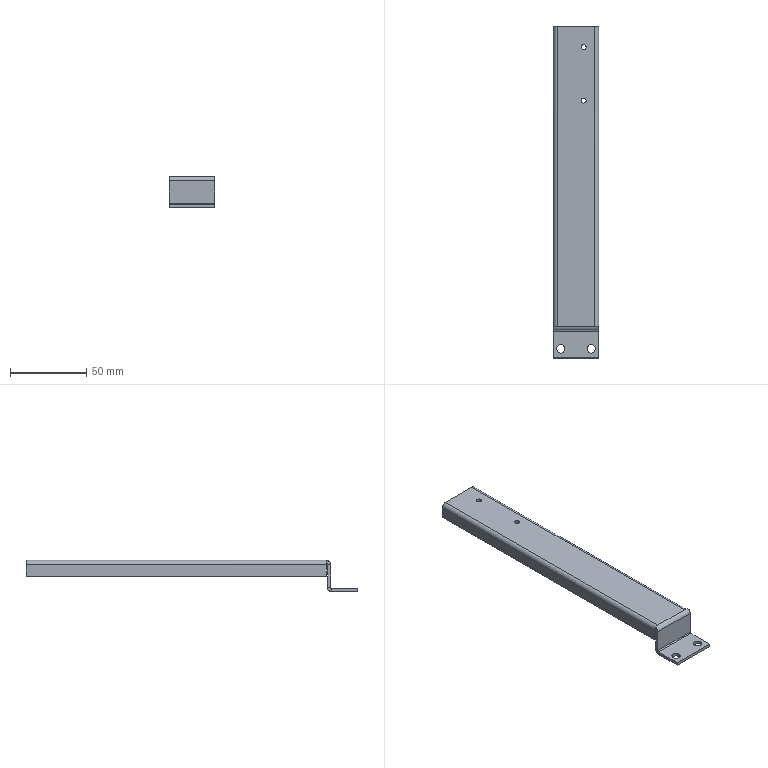Part | SolidWorks | features EdgeFlange 3, FlatPattern 1, HoleWzd 1, ICE 1, SMBaseFlange 1, SheetMetal 1 | 1 solid | 48 faces | box 30 x 218 x 20.5 mm | volume 20090 mm3 | plane 32 | cylinder 16 | commonest cylinder face diameters 1.473 x4 3.3 x4 5.473 x4 5.5 x4
STEP:
#1=CARTESIAN_POINT('',(3.35,194.,16.5));
#2=VERTEX_POINT('',#1);
#3=CARTESIAN_POINT('',(6.65,194.,16.5));
#4=VERTEX_POINT('',#3);
#5=CARTESIAN_POINT('',(5.,194.,16.5));
#6=DIRECTION('',(0.,0.,1.));
#7=DIRECTION('',(0.,-1.,0.));
#8=AXIS2_PLACEMENT_3D('',#5,#6,#7);
#9=CIRCLE('',#8,1.65);
#10=EDGE_CURVE('',#2,#4,#9,.T.);
#11=ORIENTED_EDGE('',*,*,#10,.F.);
#12=CARTESIAN_POINT('',(3.35,194.,18.5));
#13=VERTEX_POINT('',#12);
#14=CARTESIAN_POINT('',(3.35,194.,18.5));
#15=DIRECTION('',(0.,0.,1.));
#16=VECTOR('',#15,1000.);
#17=LINE('',#14,#16);
#18=EDGE_CURVE('',#2,#13,#17,.T.);
#19=ORIENTED_EDGE('',*,*,#18,.T.);
#20=CARTESIAN_POINT('',(6.65,194.,18.5));
#21=VERTEX_POINT('',#20);
#22=CARTESIAN_POINT('',(5.,194.,18.5));
#23=DIRECTION('',(0.,0.,1.));
#24=DIRECTION('',(1.,0.,0.));
#25=AXIS2_PLACEMENT_3D('',#22,#23,#24);
#26=CIRCLE('',#25,1.65);
#27=EDGE_CURVE('',#13,#21,#26,.T.);
#28=ORIENTED_EDGE('',*,*,#27,.T.);
#29=CARTESIAN_POINT('',(6.65,194.,18.5));
#30=DIRECTION('',(0.,0.,1.));
#31=VECTOR('',#30,1000.);
#32=LINE('',#29,#31);
#33=EDGE_CURVE('',#4,#21,#32,.T.);
#34=ORIENTED_EDGE('',*,*,#33,.F.);
#35=EDGE_LOOP('',(#11,#19,#28,#34));
#36=FACE_OUTER_BOUND('',#35,.T.);
#37=CARTESIAN_POINT('',(5.,194.,18.5));
#38=DIRECTION('',(0.,0.,1.));
#39=DIRECTION('',(1.,0.,0.));
#40=AXIS2_PLACEMENT_3D('',#37,#38,#39);
#41=CYLINDRICAL_SURFACE('',#40,1.65);
#42=ADVANCED_FACE('',(#36),#41,.F.);
#43=CARTESIAN_POINT('',(3.35,159.,16.5));
#44=VERTEX_POINT('',#43);
#45=CARTESIAN_POINT('',(6.65,159.,16.5));
#46=VERTEX_POINT('',#45);
#47=CARTESIAN_POINT('',(5.,159.,16.5));
#48=DIRECTION('',(0.,0.,1.));
#49=DIRECTION('',(0.,-1.,0.));
#50=AXIS2_PLACEMENT_3D('',#47,#48,#49);
#51=CIRCLE('',#50,1.65);
#52=EDGE_CURVE('',#44,#46,#51,.T.);
#53=ORIENTED_EDGE('',*,*,#52,.F.);
#54=CARTESIAN_POINT('',(3.35,159.,18.5));
#55=VERTEX_POINT('',#54);
#56=CARTESIAN_POINT('',(3.35,159.,18.5));
#57=DIRECTION('',(0.,0.,1.));
#58=VECTOR('',#57,1000.);
#59=LINE('',#56,#58);
#60=EDGE_CURVE('',#44,#55,#59,.T.);
#61=ORIENTED_EDGE('',*,*,#60,.T.);
#62=CARTESIAN_POINT('',(6.65,159.,18.5));
#63=VERTEX_POINT('',#62);
#64=CARTESIAN_POINT('',(5.,159.,18.5));
#65=DIRECTION('',(0.,0.,1.));
#66=DIRECTION('',(1.,0.,0.));
#67=AXIS2_PLACEMENT_3D('',#64,#65,#66);
#68=CIRCLE('',#67,1.65);
#69=EDGE_CURVE('',#55,#63,#68,.T.);
#70=ORIENTED_EDGE('',*,*,#69,.T.);
#71=CARTESIAN_POINT('',(6.65,159.,18.5));
#72=DIRECTION('',(0.,0.,1.));
#73=VECTOR('',#72,1000.);
#74=LINE('',#71,#73);
#75=EDGE_CURVE('',#46,#63,#74,.T.);
#76=ORIENTED_EDGE('',*,*,#75,.F.);
#77=EDGE_LOOP('',(#53,#61,#70,#76));
#78=FACE_OUTER_BOUND('',#77,.T.);
#79=CARTESIAN_POINT('',(5.,159.,18.5));
#80=DIRECTION('',(0.,0.,1.));
#81=DIRECTION('',(1.,0.,0.));
#82=AXIS2_PLACEMENT_3D('',#79,#80,#81);
#83=CYLINDRICAL_SURFACE('',#82,1.65);
#84=ADVANCED_FACE('',(#78),#83,.F.);
#85=CARTESIAN_POINT('',(7.25,-4.,-2.));
#86=VERTEX_POINT('',#85);
#87=CARTESIAN_POINT('',(12.75,-4.,-2.));
#88=VERTEX_POINT('',#87);
#89=CARTESIAN_POINT('',(10.,-4.,-2.));
#90=DIRECTION('',(0.,0.,1.));
#91=DIRECTION('',(1.,0.,0.));
#92=AXIS2_PLACEMENT_3D('',#89,#90,#91);
#93=CIRCLE('',#92,2.75);
#94=EDGE_CURVE('',#86,#88,#93,.T.);
#95=ORIENTED_EDGE('',*,*,#94,.F.);
#96=CARTESIAN_POINT('',(7.25,-4.,0.));
#97=VERTEX_POINT('',#96);
#98=CARTESIAN_POINT('',(7.25,-4.,-2.));
#99=DIRECTION('',(0.,0.,1.));
#100=VECTOR('',#99,1000.);
#101=LINE('',#98,#100);
#102=EDGE_CURVE('',#86,#97,#101,.T.);
#103=ORIENTED_EDGE('',*,*,#102,.T.);
#104=CARTESIAN_POINT('',(12.75,-4.,0.));
#105=VERTEX_POINT('',#104);
#106=CARTESIAN_POINT('',(10.,-4.,0.));
#107=DIRECTION('',(0.,0.,1.));
#108=DIRECTION('',(1.,0.,0.));
#109=AXIS2_PLACEMENT_3D('',#106,#107,#108);
#110=CIRCLE('',#109,2.75);
#111=EDGE_CURVE('',#97,#105,#110,.T.);
#112=ORIENTED_EDGE('',*,*,#111,.T.);
#113=CARTESIAN_POINT('',(12.75,-4.,-2.));
#114=DIRECTION('',(0.,0.,1.));
#115=VECTOR('',#114,1000.);
#116=LINE('',#113,#115);
#117=EDGE_CURVE('',#88,#105,#116,.T.);
#118=ORIENTED_EDGE('',*,*,#117,.F.);
#119=EDGE_LOOP('',(#95,#103,#112,#118));
#120=FACE_OUTER_BOUND('',#119,.T.);
#121=CARTESIAN_POINT('',(10.,-4.,-2.));
#122=DIRECTION('',(0.,0.,1.));
#123=DIRECTION('',(1.,0.,0.));
#124=AXIS2_PLACEMENT_3D('',#121,#122,#123);
#125=CYLINDRICAL_SURFACE('',#124,2.75);
#126=ADVANCED_FACE('',(#120),#125,.F.);
#127=CARTESIAN_POINT('',(-12.75,-4.,-2.));
#128=VERTEX_POINT('',#127);
#129=CARTESIAN_POINT('',(-7.25,-4.,-2.));
#130=VERTEX_POINT('',#129);
#131=CARTESIAN_POINT('',(-10.,-4.,-2.));
#132=DIRECTION('',(0.,0.,1.));
#133=DIRECTION('',(1.,0.,0.));
#134=AXIS2_PLACEMENT_3D('',#131,#132,#133);
#135=CIRCLE('',#134,2.75);
#136=EDGE_CURVE('',#128,#130,#135,.T.);
#137=ORIENTED_EDGE('',*,*,#136,.F.);
#138=CARTESIAN_POINT('',(-12.75,-4.,0.));
#139=VERTEX_POINT('',#138);
#140=CARTESIAN_POINT('',(-12.75,-4.,-2.));
#141=DIRECTION('',(0.,0.,1.));
#142=VECTOR('',#141,1000.);
#143=LINE('',#140,#142);
#144=EDGE_CURVE('',#128,#139,#143,.T.);
#145=ORIENTED_EDGE('',*,*,#144,.T.);
#146=CARTESIAN_POINT('',(-7.25,-4.,0.));
#147=VERTEX_POINT('',#146);
#148=CARTESIAN_POINT('',(-10.,-4.,0.));
#149=DIRECTION('',(0.,0.,1.));
#150=DIRECTION('',(1.,0.,0.));
#151=AXIS2_PLACEMENT_3D('',#148,#149,#150);
#152=CIRCLE('',#151,2.75);
#153=EDGE_CURVE('',#139,#147,#152,.T.);
#154=ORIENTED_EDGE('',*,*,#153,.T.);
#155=CARTESIAN_POINT('',(-7.25,-4.,-2.));
#156=DIRECTION('',(0.,0.,1.));
#157=VECTOR('',#156,1000.);
#158=LINE('',#155,#157);
#159=EDGE_CURVE('',#130,#147,#158,.T.);
#160=ORIENTED_EDGE('',*,*,#159,.F.);
#161=EDGE_LOOP('',(#137,#145,#154,#160));
#162=FACE_OUTER_BOUND('',#161,.T.);
#163=CARTESIAN_POINT('',(-10.,-4.,-2.));
#164=DIRECTION('',(0.,0.,1.));
#165=DIRECTION('',(1.,0.,0.));
#166=AXIS2_PLACEMENT_3D('',#163,#164,#165);
#167=CYLINDRICAL_SURFACE('',#166,2.75);
#168=ADVANCED_FACE('',(#162),#167,.F.);
#169=CARTESIAN_POINT('',(-15.,10.737,18.5));
#170=VERTEX_POINT('',#169);
#171=CARTESIAN_POINT('',(-12.263,10.737,18.5));
#172=VERTEX_POINT('',#171);
#173=CARTESIAN_POINT('',(0.,10.737,18.5));
#174=DIRECTION('',(1.,0.,0.));
#175=VECTOR('',#174,1000.);
#176=LINE('',#173,#175);
#177=EDGE_CURVE('',#170,#172,#176,.T.);
#178=ORIENTED_EDGE('',*,*,#177,.T.);
#179=CARTESIAN_POINT('',(-14.899,10.737,16.5));
#180=VERTEX_POINT('',#179);
#181=CARTESIAN_POINT('',(-12.263,10.737,15.763));
#182=DIRECTION('',(0.,-1.,0.));
#183=DIRECTION('',(0.,0.,1.));
#184=AXIS2_PLACEMENT_3D('',#181,#182,#183);
#185=CIRCLE('',#184,2.737);
#186=EDGE_CURVE('',#172,#180,#185,.T.);
#187=ORIENTED_EDGE('',*,*,#186,.T.);
#188=CARTESIAN_POINT('',(-15.,10.737,16.5));
#189=VERTEX_POINT('',#188);
#190=CARTESIAN_POINT('',(-15.,10.737,16.5));
#191=DIRECTION('',(1.,0.,0.));
#192=VECTOR('',#191,1000.);
#193=LINE('',#190,#192);
#194=EDGE_CURVE('',#189,#180,#193,.T.);
#195=ORIENTED_EDGE('',*,*,#194,.F.);
#196=CARTESIAN_POINT('',(-15.,10.737,18.5));
#197=DIRECTION('',(0.,0.,1.));
#198=VECTOR('',#197,1000.);
#199=LINE('',#196,#198);
#200=EDGE_CURVE('',#189,#170,#199,.T.);
#201=ORIENTED_EDGE('',*,*,#200,.T.);
#202=EDGE_LOOP('',(#178,#187,#195,#201));
#203=FACE_OUTER_BOUND('',#202,.T.);
#204=CARTESIAN_POINT('',(-12.263,10.737,16.5));
#205=DIRECTION('',(0.,1.,0.));
#206=DIRECTION('',(-1.,0.,0.));
#207=AXIS2_PLACEMENT_3D('',#204,#205,#206);
#208=PLANE('',#207);
#209=ADVANCED_FACE('',(#203),#208,.T.);
#210=CARTESIAN_POINT('',(15.,10.737,16.5));
#211=VERTEX_POINT('',#210);
#212=CARTESIAN_POINT('',(14.899,10.737,16.5));
#213=VERTEX_POINT('',#212);
#214=CARTESIAN_POINT('',(15.,10.737,16.5));
#215=DIRECTION('',(-1.,0.,0.));
#216=VECTOR('',#215,1000.);
#217=LINE('',#214,#216);
#218=EDGE_CURVE('',#211,#213,#217,.T.);
#219=ORIENTED_EDGE('',*,*,#218,.T.);
#220=CARTESIAN_POINT('',(12.263,10.737,18.5));
#221=VERTEX_POINT('',#220);
#222=CARTESIAN_POINT('',(12.263,10.737,15.763));
#223=DIRECTION('',(0.,-1.,0.));
#224=DIRECTION('',(0.,0.,-1.));
#225=AXIS2_PLACEMENT_3D('',#222,#223,#224);
#226=CIRCLE('',#225,2.737);
#227=EDGE_CURVE('',#213,#221,#226,.T.);
#228=ORIENTED_EDGE('',*,*,#227,.T.);
#229=CARTESIAN_POINT('',(15.,10.737,18.5));
#230=VERTEX_POINT('',#229);
#231=CARTESIAN_POINT('',(0.,10.737,18.5));
#232=DIRECTION('',(-1.,0.,0.));
#233=VECTOR('',#232,1000.);
#234=LINE('',#231,#233);
#235=EDGE_CURVE('',#230,#221,#234,.T.);
#236=ORIENTED_EDGE('',*,*,#235,.F.);
#237=CARTESIAN_POINT('',(15.,10.737,16.5));
#238=DIRECTION('',(0.,0.,1.));
#239=VECTOR('',#238,1000.);
#240=LINE('',#237,#239);
#241=EDGE_CURVE('',#211,#230,#240,.T.);
#242=ORIENTED_EDGE('',*,*,#241,.F.);
#243=EDGE_LOOP('',(#219,#228,#236,#242));
#244=FACE_OUTER_BOUND('',#243,.T.);
#245=CARTESIAN_POINT('',(15.,10.737,16.5));
#246=DIRECTION('',(0.,1.,0.));
#247=DIRECTION('',(-1.,0.,0.));
#248=AXIS2_PLACEMENT_3D('',#245,#246,#247);
#249=PLANE('',#248);
#250=ADVANCED_FACE('',(#244),#249,.T.);
#251=CARTESIAN_POINT('',(5.,194.,18.5));
#252=DIRECTION('',(0.,0.,1.));
#253=DIRECTION('',(1.,0.,0.));
#254=AXIS2_PLACEMENT_3D('',#251,#252,#253);
#255=CIRCLE('',#254,1.65);
#256=EDGE_CURVE('',#21,#13,#255,.T.);
#257=ORIENTED_EDGE('',*,*,#256,.F.);
#258=ORIENTED_EDGE('',*,*,#27,.F.);
#259=EDGE_LOOP('',(#257,#258));
#260=FACE_BOUND('',#259,.T.);
#261=CARTESIAN_POINT('',(5.,159.,18.5));
#262=DIRECTION('',(0.,0.,1.));
#263=DIRECTION('',(1.,0.,0.));
#264=AXIS2_PLACEMENT_3D('',#261,#262,#263);
#265=CIRCLE('',#264,1.65);
#266=EDGE_CURVE('',#63,#55,#265,.T.);
#267=ORIENTED_EDGE('',*,*,#266,.F.);
#268=ORIENTED_EDGE('',*,*,#69,.F.);
#269=EDGE_LOOP('',(#267,#268));
#270=FACE_BOUND('',#269,.T.);
#271=CARTESIAN_POINT('',(-12.263,208.,18.5));
#272=VERTEX_POINT('',#271);
#273=CARTESIAN_POINT('',(12.263,208.,18.5));
#274=VERTEX_POINT('',#273);
#275=CARTESIAN_POINT('',(15.,208.,18.5));
#276=DIRECTION('',(1.,0.,0.));
#277=VECTOR('',#276,1000.);
#278=LINE('',#275,#277);
#279=EDGE_CURVE('',#272,#274,#278,.T.);
#280=ORIENTED_EDGE('',*,*,#279,.F.);
#281=CARTESIAN_POINT('',(-12.263,208.,18.5));
#282=DIRECTION('',(0.,-1.,0.));
#283=VECTOR('',#282,1000.);
#284=LINE('',#281,#283);
#285=EDGE_CURVE('',#272,#172,#284,.T.);
#286=ORIENTED_EDGE('',*,*,#285,.T.);
#287=CARTESIAN_POINT('',(0.,10.737,18.5));
#288=DIRECTION('',(1.,0.,0.));
#289=VECTOR('',#288,1000.);
#290=LINE('',#287,#289);
#291=EDGE_CURVE('',#172,#221,#290,.T.);
#292=ORIENTED_EDGE('',*,*,#291,.T.);
#293=CARTESIAN_POINT('',(12.263,10.737,18.5));
#294=DIRECTION('',(0.,1.,0.));
#295=VECTOR('',#294,1000.);
#296=LINE('',#293,#295);
#297=EDGE_CURVE('',#221,#274,#296,.T.);
#298=ORIENTED_EDGE('',*,*,#297,.T.);
#299=EDGE_LOOP('',(#280,#286,#292,#298));
#300=FACE_OUTER_BOUND('',#299,.T.);
#301=CARTESIAN_POINT('',(0.,0.,18.5));
#302=DIRECTION('',(0.,0.,1.));
#303=DIRECTION('',(0.,-1.,0.));
#304=AXIS2_PLACEMENT_3D('',#301,#302,#303);
#305=PLANE('',#304);
#306=ADVANCED_FACE('',(#260,#270,#300),#305,.T.);
#307=CARTESIAN_POINT('',(5.,194.,16.5));
#308=DIRECTION('',(0.,0.,1.));
#309=DIRECTION('',(0.,-1.,0.));
#310=AXIS2_PLACEMENT_3D('',#307,#308,#309);
#311=CIRCLE('',#310,1.65);
#312=EDGE_CURVE('',#4,#2,#311,.T.);
#313=ORIENTED_EDGE('',*,*,#312,.T.);
#314=ORIENTED_EDGE('',*,*,#10,.T.);
#315=EDGE_LOOP('',(#313,#314));
#316=FACE_BOUND('',#315,.T.);
#317=CARTESIAN_POINT('',(5.,159.,16.5));
#318=DIRECTION('',(0.,0.,1.));
#319=DIRECTION('',(0.,-1.,0.));
#320=AXIS2_PLACEMENT_3D('',#317,#318,#319);
#321=CIRCLE('',#320,1.65);
#322=EDGE_CURVE('',#46,#44,#321,.T.);
#323=ORIENTED_EDGE('',*,*,#322,.T.);
#324=ORIENTED_EDGE('',*,*,#52,.T.);
#325=EDGE_LOOP('',(#323,#324));
#326=FACE_BOUND('',#325,.T.);
#327=CARTESIAN_POINT('',(-12.263,208.,16.5));
#328=VERTEX_POINT('',#327);
#329=CARTESIAN_POINT('',(-12.263,10.737,16.5));
#330=VERTEX_POINT('',#329);
#331=CARTESIAN_POINT('',(-12.263,208.,16.5));
#332=DIRECTION('',(0.,-1.,0.));
#333=VECTOR('',#332,1000.);
#334=LINE('',#331,#333);
#335=EDGE_CURVE('',#328,#330,#334,.T.);
#336=ORIENTED_EDGE('',*,*,#335,.F.);
#337=CARTESIAN_POINT('',(12.263,208.,16.5));
#338=VERTEX_POINT('',#337);
#339=CARTESIAN_POINT('',(0.,208.,16.5));
#340=DIRECTION('',(1.,0.,0.));
#341=VECTOR('',#340,1000.);
#342=LINE('',#339,#341);
#343=EDGE_CURVE('',#328,#338,#342,.T.);
#344=ORIENTED_EDGE('',*,*,#343,.T.);
#345=CARTESIAN_POINT('',(12.263,10.737,16.5));
#346=VERTEX_POINT('',#345);
#347=CARTESIAN_POINT('',(12.263,10.737,16.5));
#348=DIRECTION('',(0.,1.,0.));
#349=VECTOR('',#348,1000.);
#350=LINE('',#347,#349);
#351=EDGE_CURVE('',#346,#338,#350,.T.);
#352=ORIENTED_EDGE('',*,*,#351,.F.);
#353=CARTESIAN_POINT('',(-15.,10.737,16.5));
#354=DIRECTION('',(1.,0.,0.));
#355=VECTOR('',#354,1000.);
#356=LINE('',#353,#355);
#357=EDGE_CURVE('',#330,#346,#356,.T.);
#358=ORIENTED_EDGE('',*,*,#357,.F.);
#359=EDGE_LOOP('',(#336,#344,#352,#358));
#360=FACE_OUTER_BOUND('',#359,.T.);
#361=CARTESIAN_POINT('',(0.,0.,16.5));
#362=DIRECTION('',(0.,0.,1.));
#363=DIRECTION('',(0.,-1.,0.));
#364=AXIS2_PLACEMENT_3D('',#361,#362,#363);
#365=PLANE('',#364);
#366=ADVANCED_FACE('',(#316,#326,#360),#365,.F.);
#367=ORIENTED_EDGE('',*,*,#343,.F.);
#368=CARTESIAN_POINT('',(-12.263,208.,16.5));
#369=DIRECTION('',(0.,0.,1.));
#370=VECTOR('',#369,1000.);
#371=LINE('',#368,#370);
#372=EDGE_CURVE('',#328,#272,#371,.T.);
#373=ORIENTED_EDGE('',*,*,#372,.T.);
#374=ORIENTED_EDGE('',*,*,#279,.T.);
#375=CARTESIAN_POINT('',(12.263,208.,16.5));
#376=DIRECTION('',(0.,0.,1.));
#377=VECTOR('',#376,1000.);
#378=LINE('',#375,#377);
#379=EDGE_CURVE('',#338,#274,#378,.T.);
#380=ORIENTED_EDGE('',*,*,#379,.F.);
#381=EDGE_LOOP('',(#367,#373,#374,#380));
#382=FACE_OUTER_BOUND('',#381,.T.);
#383=CARTESIAN_POINT('',(15.,208.,18.5));
#384=DIRECTION('',(0.,1.,0.));
#385=DIRECTION('',(0.,0.,1.));
#386=AXIS2_PLACEMENT_3D('',#383,#384,#385);
#387=PLANE('',#386);
#388=ADVANCED_FACE('',(#382),#387,.T.);
#389=CARTESIAN_POINT('',(15.,10.,0.7366));
#390=VERTEX_POINT('',#389);
#391=CARTESIAN_POINT('',(15.,10.,15.763));
#392=VERTEX_POINT('',#391);
#393=CARTESIAN_POINT('',(15.,10.,18.5));
#394=DIRECTION('',(0.,0.,1.));
#395=VECTOR('',#394,1000.);
#396=LINE('',#393,#395);
#397=EDGE_CURVE('',#390,#392,#396,.T.);
#398=ORIENTED_EDGE('',*,*,#397,.T.);
#399=CARTESIAN_POINT('',(15.,8.,15.763));
#400=VERTEX_POINT('',#399);
#401=CARTESIAN_POINT('',(15.,10.,15.763));
#402=DIRECTION('',(0.,-1.,0.));
#403=VECTOR('',#402,1000.);
#404=LINE('',#401,#403);
#405=EDGE_CURVE('',#392,#400,#404,.T.);
#406=ORIENTED_EDGE('',*,*,#405,.T.);
#407=CARTESIAN_POINT('',(15.,8.,0.7366));
#408=VERTEX_POINT('',#407);
#409=CARTESIAN_POINT('',(15.,8.,0.));
#410=DIRECTION('',(0.,0.,1.));
#411=VECTOR('',#410,1000.);
#412=LINE('',#409,#411);
#413=EDGE_CURVE('',#408,#400,#412,.T.);
#414=ORIENTED_EDGE('',*,*,#413,.F.);
#415=CARTESIAN_POINT('',(15.,10.,0.7366));
#416=DIRECTION('',(0.,1.,0.));
#417=VECTOR('',#416,1000.);
#418=LINE('',#415,#417);
#419=EDGE_CURVE('',#408,#390,#418,.T.);
#420=ORIENTED_EDGE('',*,*,#419,.T.);
#421=EDGE_LOOP('',(#398,#406,#414,#420));
#422=FACE_OUTER_BOUND('',#421,.T.);
#423=CARTESIAN_POINT('',(15.,10.,18.5));
#424=DIRECTION('',(1.,0.,0.));
#425=DIRECTION('',(0.,1.,0.));
#426=AXIS2_PLACEMENT_3D('',#423,#424,#425);
#427=PLANE('',#426);
#428=ADVANCED_FACE('',(#422),#427,.T.);
#429=CARTESIAN_POINT('',(-15.,10.,15.763));
#430=VERTEX_POINT('',#429);
#431=CARTESIAN_POINT('',(-15.,10.,0.7366));
#432=VERTEX_POINT('',#431);
#433=CARTESIAN_POINT('',(-15.,10.,0.));
#434=DIRECTION('',(0.,0.,-1.));
#435=VECTOR('',#434,1000.);
#436=LINE('',#433,#435);
#437=EDGE_CURVE('',#430,#432,#436,.T.);
#438=ORIENTED_EDGE('',*,*,#437,.F.);
#439=CARTESIAN_POINT('',(15.,10.,15.763));
#440=DIRECTION('',(-1.,0.,0.));
#441=VECTOR('',#440,1000.);
#442=LINE('',#439,#441);
#443=EDGE_CURVE('',#392,#430,#442,.T.);
#444=ORIENTED_EDGE('',*,*,#443,.F.);
#445=ORIENTED_EDGE('',*,*,#397,.F.);
#446=CARTESIAN_POINT('',(0.,10.,0.7366));
#447=DIRECTION('',(-1.,0.,0.));
#448=VECTOR('',#447,1000.);
#449=LINE('',#446,#448);
#450=EDGE_CURVE('',#390,#432,#449,.T.);
#451=ORIENTED_EDGE('',*,*,#450,.T.);
#452=EDGE_LOOP('',(#438,#444,#445,#451));
#453=FACE_OUTER_BOUND('',#452,.T.);
#454=CARTESIAN_POINT('',(0.,10.,0.));
#455=DIRECTION('',(0.,1.,0.));
#456=DIRECTION('',(0.,0.,1.));
#457=AXIS2_PLACEMENT_3D('',#454,#455,#456);
#458=PLANE('',#457);
#459=ADVANCED_FACE('',(#453),#458,.T.);
#460=CARTESIAN_POINT('',(-15.,8.,15.763));
#461=VERTEX_POINT('',#460);
#462=CARTESIAN_POINT('',(15.,8.,15.763));
#463=DIRECTION('',(-1.,0.,0.));
#464=VECTOR('',#463,1000.);
#465=LINE('',#462,#464);
#466=EDGE_CURVE('',#400,#461,#465,.T.);
#467=ORIENTED_EDGE('',*,*,#466,.T.);
#468=CARTESIAN_POINT('',(-15.,8.,0.7366));
#469=VERTEX_POINT('',#468);
#470=CARTESIAN_POINT('',(-15.,8.,0.));
#471=DIRECTION('',(0.,0.,-1.));
#472=VECTOR('',#471,1000.);
#473=LINE('',#470,#472);
#474=EDGE_CURVE('',#461,#469,#473,.T.);
#475=ORIENTED_EDGE('',*,*,#474,.T.);
#476=CARTESIAN_POINT('',(15.,8.,0.7366));
#477=DIRECTION('',(-1.,0.,0.));
#478=VECTOR('',#477,1000.);
#479=LINE('',#476,#478);
#480=EDGE_CURVE('',#408,#469,#479,.T.);
#481=ORIENTED_EDGE('',*,*,#480,.F.);
#482=ORIENTED_EDGE('',*,*,#413,.T.);
#483=EDGE_LOOP('',(#467,#475,#481,#482));
#484=FACE_OUTER_BOUND('',#483,.T.);
#485=CARTESIAN_POINT('',(0.,8.,0.));
#486=DIRECTION('',(0.,1.,0.));
#487=DIRECTION('',(0.,0.,1.));
#488=AXIS2_PLACEMENT_3D('',#485,#486,#487);
#489=PLANE('',#488);
#490=ADVANCED_FACE('',(#484),#489,.F.);
#491=CARTESIAN_POINT('',(-15.,7.263,0.));
#492=VERTEX_POINT('',#491);
#493=CARTESIAN_POINT('',(-15.,-10.,0.));
#494=VERTEX_POINT('',#493);
#495=CARTESIAN_POINT('',(-15.,-10.,0.));
#496=DIRECTION('',(0.,-1.,0.));
#497=VECTOR('',#496,1000.);
#498=LINE('',#495,#497);
#499=EDGE_CURVE('',#492,#494,#498,.T.);
#500=ORIENTED_EDGE('',*,*,#499,.F.);
#501=CARTESIAN_POINT('',(-15.,7.263,-2.));
#502=VERTEX_POINT('',#501);
#503=CARTESIAN_POINT('',(-15.,7.263,0.));
#504=DIRECTION('',(0.,0.,-1.));
#505=VECTOR('',#504,1000.);
#506=LINE('',#503,#505);
#507=EDGE_CURVE('',#492,#502,#506,.T.);
#508=ORIENTED_EDGE('',*,*,#507,.T.);
#509=CARTESIAN_POINT('',(-15.,-10.,-2.));
#510=VERTEX_POINT('',#509);
#511=CARTESIAN_POINT('',(-15.,-10.,-2.));
#512=DIRECTION('',(0.,-1.,0.));
#513=VECTOR('',#512,1000.);
#514=LINE('',#511,#513);
#515=EDGE_CURVE('',#502,#510,#514,.T.);
#516=ORIENTED_EDGE('',*,*,#515,.T.);
#517=CARTESIAN_POINT('',(-15.,-10.,-2.));
#518=DIRECTION('',(0.,0.,1.));
#519=VECTOR('',#518,1000.);
#520=LINE('',#517,#519);
#521=EDGE_CURVE('',#510,#494,#520,.T.);
#522=ORIENTED_EDGE('',*,*,#521,.T.);
#523=EDGE_LOOP('',(#500,#508,#516,#522));
#524=FACE_OUTER_BOUND('',#523,.T.);
#525=CARTESIAN_POINT('',(-15.,-10.,-2.));
#526=DIRECTION('',(-1.,0.,0.));
#527=DIRECTION('',(0.,0.,1.));
#528=AXIS2_PLACEMENT_3D('',#525,#526,#527);
#529=PLANE('',#528);
#530=ADVANCED_FACE('',(#524),#529,.T.);
#531=CARTESIAN_POINT('',(10.,-4.,-2.));
#532=DIRECTION('',(0.,0.,1.));
#533=DIRECTION('',(1.,0.,0.));
#534=AXIS2_PLACEMENT_3D('',#531,#532,#533);
#535=CIRCLE('',#534,2.75);
#536=EDGE_CURVE('',#88,#86,#535,.T.);
#537=ORIENTED_EDGE('',*,*,#536,.T.);
#538=ORIENTED_EDGE('',*,*,#94,.T.);
#539=EDGE_LOOP('',(#537,#538));
#540=FACE_BOUND('',#539,.T.);
#541=CARTESIAN_POINT('',(-10.,-4.,-2.));
#542=DIRECTION('',(0.,0.,1.));
#543=DIRECTION('',(1.,0.,0.));
#544=AXIS2_PLACEMENT_3D('',#541,#542,#543);
#545=CIRCLE('',#544,2.75);
#546=EDGE_CURVE('',#130,#128,#545,.T.);
#547=ORIENTED_EDGE('',*,*,#546,.T.);
#548=ORIENTED_EDGE('',*,*,#136,.T.);
#549=EDGE_LOOP('',(#547,#548));
#550=FACE_BOUND('',#549,.T.);
#551=CARTESIAN_POINT('',(15.,7.263,-2.));
#552=VERTEX_POINT('',#551);
#553=CARTESIAN_POINT('',(-15.,7.263,-2.));
#554=DIRECTION('',(1.,0.,0.));
#555=VECTOR('',#554,1000.);
#556=LINE('',#553,#555);
#557=EDGE_CURVE('',#502,#552,#556,.T.);
#558=ORIENTED_EDGE('',*,*,#557,.T.);
#559=CARTESIAN_POINT('',(15.,-10.,-2.));
#560=VERTEX_POINT('',#559);
#561=CARTESIAN_POINT('',(15.,-10.,-2.));
#562=DIRECTION('',(0.,1.,0.));
#563=VECTOR('',#562,1000.);
#564=LINE('',#561,#563);
#565=EDGE_CURVE('',#560,#552,#564,.T.);
#566=ORIENTED_EDGE('',*,*,#565,.F.);
#567=CARTESIAN_POINT('',(15.,-10.,-2.));
#568=DIRECTION('',(1.,0.,0.));
#569=VECTOR('',#568,1000.);
#570=LINE('',#567,#569);
#571=EDGE_CURVE('',#510,#560,#570,.T.);
#572=ORIENTED_EDGE('',*,*,#571,.F.);
#573=ORIENTED_EDGE('',*,*,#515,.F.);
#574=EDGE_LOOP('',(#558,#566,#572,#573));
#575=FACE_OUTER_BOUND('',#574,.T.);
#576=CARTESIAN_POINT('',(0.,0.,-2.));
#577=DIRECTION('',(0.,0.,1.));
#578=DIRECTION('',(1.,0.,0.));
#579=AXIS2_PLACEMENT_3D('',#576,#577,#578);
#580=PLANE('',#579);
#581=ADVANCED_FACE('',(#540,#550,#575),#580,.F.);
#582=CARTESIAN_POINT('',(10.,-4.,0.));
#583=DIRECTION('',(0.,0.,1.));
#584=DIRECTION('',(1.,0.,0.));
#585=AXIS2_PLACEMENT_3D('',#582,#583,#584);
#586=CIRCLE('',#585,2.75);
#587=EDGE_CURVE('',#105,#97,#586,.T.);
#588=ORIENTED_EDGE('',*,*,#587,.F.);
#589=ORIENTED_EDGE('',*,*,#111,.F.);
#590=EDGE_LOOP('',(#588,#589));
#591=FACE_BOUND('',#590,.T.);
#592=CARTESIAN_POINT('',(-10.,-4.,0.));
#593=DIRECTION('',(0.,0.,1.));
#594=DIRECTION('',(1.,0.,0.));
#595=AXIS2_PLACEMENT_3D('',#592,#593,#594);
#596=CIRCLE('',#595,2.75);
#597=EDGE_CURVE('',#147,#139,#596,.T.);
#598=ORIENTED_EDGE('',*,*,#597,.F.);
#599=ORIENTED_EDGE('',*,*,#153,.F.);
#600=EDGE_LOOP('',(#598,#599));
#601=FACE_BOUND('',#600,.T.);
#602=CARTESIAN_POINT('',(15.,-10.,0.));
#603=VERTEX_POINT('',#602);
#604=CARTESIAN_POINT('',(15.,7.263,0.));
#605=VERTEX_POINT('',#604);
#606=CARTESIAN_POINT('',(15.,-10.,0.));
#607=DIRECTION('',(0.,1.,0.));
#608=VECTOR('',#607,1000.);
#609=LINE('',#606,#608);
#610=EDGE_CURVE('',#603,#605,#609,.T.);
#611=ORIENTED_EDGE('',*,*,#610,.T.);
#612=CARTESIAN_POINT('',(-15.,7.263,0.));
#613=DIRECTION('',(1.,0.,0.));
#614=VECTOR('',#613,1000.);
#615=LINE('',#612,#614);
#616=EDGE_CURVE('',#492,#605,#615,.T.);
#617=ORIENTED_EDGE('',*,*,#616,.F.);
#618=ORIENTED_EDGE('',*,*,#499,.T.);
#619=CARTESIAN_POINT('',(15.,-10.,0.));
#620=DIRECTION('',(1.,0.,0.));
#621=VECTOR('',#620,1000.);
#622=LINE('',#619,#621);
#623=EDGE_CURVE('',#494,#603,#622,.T.);
#624=ORIENTED_EDGE('',*,*,#623,.T.);
#625=EDGE_LOOP('',(#611,#617,#618,#624));
#626=FACE_OUTER_BOUND('',#625,.T.);
#627=CARTESIAN_POINT('',(0.,0.,0.));
#628=DIRECTION('',(0.,0.,1.));
#629=DIRECTION('',(1.,0.,0.));
#630=AXIS2_PLACEMENT_3D('',#627,#628,#629);
#631=PLANE('',#630);
#632=ADVANCED_FACE('',(#591,#601,#626),#631,.T.);
#633=CARTESIAN_POINT('',(15.,7.263,0.));
#634=DIRECTION('',(0.,0.,-1.));
#635=VECTOR('',#634,1000.);
#636=LINE('',#633,#635);
#637=EDGE_CURVE('',#605,#552,#636,.T.);
#638=ORIENTED_EDGE('',*,*,#637,.F.);
#639=ORIENTED_EDGE('',*,*,#610,.F.);
#640=CARTESIAN_POINT('',(15.,-10.,-2.));
#641=DIRECTION('',(0.,0.,1.));
#642=VECTOR('',#641,1000.);
#643=LINE('',#640,#642);
#644=EDGE_CURVE('',#560,#603,#643,.T.);
#645=ORIENTED_EDGE('',*,*,#644,.F.);
#646=ORIENTED_EDGE('',*,*,#565,.T.);
#647=EDGE_LOOP('',(#638,#639,#645,#646));
#648=FACE_OUTER_BOUND('',#647,.T.);
#649=CARTESIAN_POINT('',(15.,-10.,-2.));
#650=DIRECTION('',(1.,0.,0.));
#651=DIRECTION('',(0.,0.,-1.));
#652=AXIS2_PLACEMENT_3D('',#649,#650,#651);
#653=PLANE('',#652);
#654=ADVANCED_FACE('',(#648),#653,.T.);
#655=ORIENTED_EDGE('',*,*,#623,.F.);
#656=ORIENTED_EDGE('',*,*,#521,.F.);
#657=ORIENTED_EDGE('',*,*,#571,.T.);
#658=ORIENTED_EDGE('',*,*,#644,.T.);
#659=EDGE_LOOP('',(#655,#656,#657,#658));
#660=FACE_OUTER_BOUND('',#659,.T.);
#661=CARTESIAN_POINT('',(15.,-10.,-2.));
#662=DIRECTION('',(0.,-1.,0.));
#663=DIRECTION('',(1.,0.,0.));
#664=AXIS2_PLACEMENT_3D('',#661,#662,#663);
#665=PLANE('',#664);
#666=ADVANCED_FACE('',(#660),#665,.T.);
#667=ORIENTED_EDGE('',*,*,#419,.F.);
#668=CARTESIAN_POINT('',(15.,7.263,0.7366));
#669=DIRECTION('',(1.,0.,0.));
#670=DIRECTION('',(0.,0.,1.));
#671=AXIS2_PLACEMENT_3D('',#668,#669,#670);
#672=CIRCLE('',#671,0.7366);
#673=EDGE_CURVE('',#605,#408,#672,.T.);
#674=ORIENTED_EDGE('',*,*,#673,.F.);
#675=ORIENTED_EDGE('',*,*,#637,.T.);
#676=CARTESIAN_POINT('',(15.,7.263,0.7366));
#677=DIRECTION('',(1.,0.,0.));
#678=DIRECTION('',(0.,0.,1.));
#679=AXIS2_PLACEMENT_3D('',#676,#677,#678);
#680=CIRCLE('',#679,2.737);
#681=EDGE_CURVE('',#552,#390,#680,.T.);
#682=ORIENTED_EDGE('',*,*,#681,.T.);
#683=EDGE_LOOP('',(#667,#674,#675,#682));
#684=FACE_OUTER_BOUND('',#683,.T.);
#685=CARTESIAN_POINT('',(15.,7.263,0.7366));
#686=DIRECTION('',(1.,0.,0.));
#687=DIRECTION('',(0.,0.,-1.));
#688=AXIS2_PLACEMENT_3D('',#685,#686,#687);
#689=PLANE('',#688);
#690=ADVANCED_FACE('',(#684),#689,.T.);
#691=CARTESIAN_POINT('',(-15.,7.263,0.7366));
#692=DIRECTION('',(-1.,0.,0.));
#693=DIRECTION('',(0.,0.,1.));
#694=AXIS2_PLACEMENT_3D('',#691,#692,#693);
#695=CIRCLE('',#694,0.7366);
#696=EDGE_CURVE('',#469,#492,#695,.T.);
#697=ORIENTED_EDGE('',*,*,#696,.F.);
#698=CARTESIAN_POINT('',(-15.,8.,0.7366));
#699=DIRECTION('',(0.,1.,0.));
#700=VECTOR('',#699,1000.);
#701=LINE('',#698,#700);
#702=EDGE_CURVE('',#469,#432,#701,.T.);
#703=ORIENTED_EDGE('',*,*,#702,.T.);
#704=CARTESIAN_POINT('',(-15.,7.263,0.7366));
#705=DIRECTION('',(-1.,0.,0.));
#706=DIRECTION('',(0.,0.,1.));
#707=AXIS2_PLACEMENT_3D('',#704,#705,#706);
#708=CIRCLE('',#707,2.737);
#709=EDGE_CURVE('',#432,#502,#708,.T.);
#710=ORIENTED_EDGE('',*,*,#709,.T.);
#711=ORIENTED_EDGE('',*,*,#507,.F.);
#712=EDGE_LOOP('',(#697,#703,#710,#711));
#713=FACE_OUTER_BOUND('',#712,.T.);
#714=CARTESIAN_POINT('',(-15.,7.263,0.7366));
#715=DIRECTION('',(1.,0.,0.));
#716=DIRECTION('',(0.,0.,-1.));
#717=AXIS2_PLACEMENT_3D('',#714,#715,#716);
#718=PLANE('',#717);
#719=ADVANCED_FACE('',(#713),#718,.F.);
#720=ORIENTED_EDGE('',*,*,#557,.F.);
#721=ORIENTED_EDGE('',*,*,#709,.F.);
#722=ORIENTED_EDGE('',*,*,#450,.F.);
#723=ORIENTED_EDGE('',*,*,#681,.F.);
#724=EDGE_LOOP('',(#720,#721,#722,#723));
#725=FACE_OUTER_BOUND('',#724,.T.);
#726=CARTESIAN_POINT('',(-15.,7.263,0.7366));
#727=DIRECTION('',(-1.,0.,0.));
#728=DIRECTION('',(0.,1.,0.));
#729=AXIS2_PLACEMENT_3D('',#726,#727,#728);
#730=CYLINDRICAL_SURFACE('',#729,2.737);
#731=ADVANCED_FACE('',(#725),#730,.T.);
#732=ORIENTED_EDGE('',*,*,#616,.T.);
#733=ORIENTED_EDGE('',*,*,#673,.T.);
#734=ORIENTED_EDGE('',*,*,#480,.T.);
#735=ORIENTED_EDGE('',*,*,#696,.T.);
#736=EDGE_LOOP('',(#732,#733,#734,#735));
#737=FACE_OUTER_BOUND('',#736,.T.);
#738=CARTESIAN_POINT('',(-15.,7.263,0.7366));
#739=DIRECTION('',(-1.,0.,0.));
#740=DIRECTION('',(0.,1.,0.));
#741=AXIS2_PLACEMENT_3D('',#738,#739,#740);
#742=CYLINDRICAL_SURFACE('',#741,0.7366);
#743=ADVANCED_FACE('',(#737),#742,.F.);
#744=CARTESIAN_POINT('',(-15.,10.,15.763));
#745=DIRECTION('',(0.,-1.,0.));
#746=VECTOR('',#745,1000.);
#747=LINE('',#744,#746);
#748=EDGE_CURVE('',#430,#461,#747,.T.);
#749=ORIENTED_EDGE('',*,*,#748,.F.);
#750=ORIENTED_EDGE('',*,*,#437,.T.);
#751=ORIENTED_EDGE('',*,*,#702,.F.);
#752=ORIENTED_EDGE('',*,*,#474,.F.);
#753=EDGE_LOOP('',(#749,#750,#751,#752));
#754=FACE_OUTER_BOUND('',#753,.T.);
#755=CARTESIAN_POINT('',(-15.,10.,0.));
#756=DIRECTION('',(-1.,0.,0.));
#757=DIRECTION('',(0.,-1.,0.));
#758=AXIS2_PLACEMENT_3D('',#755,#756,#757);
#759=PLANE('',#758);
#760=ADVANCED_FACE('',(#754),#759,.T.);
#761=ORIENTED_EDGE('',*,*,#200,.F.);
#762=CARTESIAN_POINT('',(-15.,10.737,15.763));
#763=DIRECTION('',(-1.,0.,0.));
#764=DIRECTION('',(0.,0.,-1.));
#765=AXIS2_PLACEMENT_3D('',#762,#763,#764);
#766=CIRCLE('',#765,0.7366);
#767=EDGE_CURVE('',#430,#189,#766,.T.);
#768=ORIENTED_EDGE('',*,*,#767,.F.);
#769=ORIENTED_EDGE('',*,*,#748,.T.);
#770=CARTESIAN_POINT('',(-15.,10.737,15.763));
#771=DIRECTION('',(-1.,0.,0.));
#772=DIRECTION('',(0.,0.,-1.));
#773=AXIS2_PLACEMENT_3D('',#770,#771,#772);
#774=CIRCLE('',#773,2.737);
#775=EDGE_CURVE('',#461,#170,#774,.T.);
#776=ORIENTED_EDGE('',*,*,#775,.T.);
#777=EDGE_LOOP('',(#761,#768,#769,#776));
#778=FACE_OUTER_BOUND('',#777,.T.);
#779=CARTESIAN_POINT('',(-15.,10.737,15.763));
#780=DIRECTION('',(-1.,0.,0.));
#781=DIRECTION('',(0.,0.,1.));
#782=AXIS2_PLACEMENT_3D('',#779,#780,#781);
#783=PLANE('',#782);
#784=ADVANCED_FACE('',(#778),#783,.T.);
#785=CARTESIAN_POINT('',(15.,10.737,15.763));
#786=DIRECTION('',(1.,0.,0.));
#787=DIRECTION('',(0.,0.,-1.));
#788=AXIS2_PLACEMENT_3D('',#785,#786,#787);
#789=CIRCLE('',#788,0.7366);
#790=EDGE_CURVE('',#211,#392,#789,.T.);
#791=ORIENTED_EDGE('',*,*,#790,.F.);
#792=ORIENTED_EDGE('',*,*,#241,.T.);
#793=CARTESIAN_POINT('',(15.,10.737,15.763));
#794=DIRECTION('',(1.,0.,0.));
#795=DIRECTION('',(0.,0.,-1.));
#796=AXIS2_PLACEMENT_3D('',#793,#794,#795);
#797=CIRCLE('',#796,2.737);
#798=EDGE_CURVE('',#230,#400,#797,.T.);
#799=ORIENTED_EDGE('',*,*,#798,.T.);
#800=ORIENTED_EDGE('',*,*,#405,.F.);
#801=EDGE_LOOP('',(#791,#792,#799,#800));
#802=FACE_OUTER_BOUND('',#801,.T.);
#803=CARTESIAN_POINT('',(15.,10.737,15.763));
#804=DIRECTION('',(-1.,0.,0.));
#805=DIRECTION('',(0.,0.,1.));
#806=AXIS2_PLACEMENT_3D('',#803,#804,#805);
#807=PLANE('',#806);
#808=ADVANCED_FACE('',(#802),#807,.F.);
#809=ORIENTED_EDGE('',*,*,#466,.F.);
#810=ORIENTED_EDGE('',*,*,#798,.F.);
#811=ORIENTED_EDGE('',*,*,#235,.T.);
#812=ORIENTED_EDGE('',*,*,#291,.F.);
#813=ORIENTED_EDGE('',*,*,#177,.F.);
#814=ORIENTED_EDGE('',*,*,#775,.F.);
#815=EDGE_LOOP('',(#809,#810,#811,#812,#813,#814));
#816=FACE_OUTER_BOUND('',#815,.T.);
#817=CARTESIAN_POINT('',(15.,10.737,15.763));
#818=DIRECTION('',(1.,0.,0.));
#819=DIRECTION('',(0.,0.,1.));
#820=AXIS2_PLACEMENT_3D('',#817,#818,#819);
#821=CYLINDRICAL_SURFACE('',#820,2.737);
#822=ADVANCED_FACE('',(#816),#821,.T.);
#823=ORIENTED_EDGE('',*,*,#443,.T.);
#824=ORIENTED_EDGE('',*,*,#767,.T.);
#825=ORIENTED_EDGE('',*,*,#194,.T.);
#826=CARTESIAN_POINT('',(-15.,10.737,16.5));
#827=DIRECTION('',(1.,0.,0.));
#828=VECTOR('',#827,1000.);
#829=LINE('',#826,#828);
#830=EDGE_CURVE('',#180,#330,#829,.T.);
#831=ORIENTED_EDGE('',*,*,#830,.T.);
#832=ORIENTED_EDGE('',*,*,#357,.T.);
#833=CARTESIAN_POINT('',(15.,10.737,16.5));
#834=DIRECTION('',(-1.,0.,0.));
#835=VECTOR('',#834,1000.);
#836=LINE('',#833,#835);
#837=EDGE_CURVE('',#213,#346,#836,.T.);
#838=ORIENTED_EDGE('',*,*,#837,.F.);
#839=ORIENTED_EDGE('',*,*,#218,.F.);
#840=ORIENTED_EDGE('',*,*,#790,.T.);
#841=EDGE_LOOP('',(#823,#824,#825,#831,#832,#838,#839,#840));
#842=FACE_OUTER_BOUND('',#841,.T.);
#843=CARTESIAN_POINT('',(15.,10.737,15.763));
#844=DIRECTION('',(1.,0.,0.));
#845=DIRECTION('',(0.,0.,1.));
#846=AXIS2_PLACEMENT_3D('',#843,#844,#845);
#847=CYLINDRICAL_SURFACE('',#846,0.7366);
#848=ADVANCED_FACE('',(#842),#847,.F.);
#849=ORIENTED_EDGE('',*,*,#144,.F.);
#850=ORIENTED_EDGE('',*,*,#546,.F.);
#851=ORIENTED_EDGE('',*,*,#159,.T.);
#852=ORIENTED_EDGE('',*,*,#597,.T.);
#853=EDGE_LOOP('',(#849,#850,#851,#852));
#854=FACE_OUTER_BOUND('',#853,.T.);
#855=CARTESIAN_POINT('',(-10.,-4.,-2.));
#856=DIRECTION('',(0.,0.,1.));
#857=DIRECTION('',(1.,0.,0.));
#858=AXIS2_PLACEMENT_3D('',#855,#856,#857);
#859=CYLINDRICAL_SURFACE('',#858,2.75);
#860=ADVANCED_FACE('',(#854),#859,.F.);
#861=ORIENTED_EDGE('',*,*,#102,.F.);
#862=ORIENTED_EDGE('',*,*,#536,.F.);
#863=ORIENTED_EDGE('',*,*,#117,.T.);
#864=ORIENTED_EDGE('',*,*,#587,.T.);
#865=EDGE_LOOP('',(#861,#862,#863,#864));
#866=FACE_OUTER_BOUND('',#865,.T.);
#867=CARTESIAN_POINT('',(10.,-4.,-2.));
#868=DIRECTION('',(0.,0.,1.));
#869=DIRECTION('',(1.,0.,0.));
#870=AXIS2_PLACEMENT_3D('',#867,#868,#869);
#871=CYLINDRICAL_SURFACE('',#870,2.75);
#872=ADVANCED_FACE('',(#866),#871,.F.);
#873=ORIENTED_EDGE('',*,*,#60,.F.);
#874=ORIENTED_EDGE('',*,*,#322,.F.);
#875=ORIENTED_EDGE('',*,*,#75,.T.);
#876=ORIENTED_EDGE('',*,*,#266,.T.);
#877=EDGE_LOOP('',(#873,#874,#875,#876));
#878=FACE_OUTER_BOUND('',#877,.T.);
#879=CARTESIAN_POINT('',(5.,159.,18.5));
#880=DIRECTION('',(0.,0.,1.));
#881=DIRECTION('',(1.,0.,0.));
#882=AXIS2_PLACEMENT_3D('',#879,#880,#881);
#883=CYLINDRICAL_SURFACE('',#882,1.65);
#884=ADVANCED_FACE('',(#878),#883,.F.);
#885=ORIENTED_EDGE('',*,*,#18,.F.);
#886=ORIENTED_EDGE('',*,*,#312,.F.);
#887=ORIENTED_EDGE('',*,*,#33,.T.);
#888=ORIENTED_EDGE('',*,*,#256,.T.);
#889=EDGE_LOOP('',(#885,#886,#887,#888));
#890=FACE_OUTER_BOUND('',#889,.T.);
#891=CARTESIAN_POINT('',(5.,194.,18.5));
#892=DIRECTION('',(0.,0.,1.));
#893=DIRECTION('',(1.,0.,0.));
#894=AXIS2_PLACEMENT_3D('',#891,#892,#893);
#895=CYLINDRICAL_SURFACE('',#894,1.65);
#896=ADVANCED_FACE('',(#890),#895,.F.);
#897=CARTESIAN_POINT('',(13.,208.,15.763));
#898=VERTEX_POINT('',#897);
#899=CARTESIAN_POINT('',(15.,208.,15.763));
#900=VERTEX_POINT('',#899);
#901=CARTESIAN_POINT('',(15.,208.,15.763));
#902=DIRECTION('',(1.,0.,0.));
#903=VECTOR('',#902,1000.);
#904=LINE('',#901,#903);
#905=EDGE_CURVE('',#898,#900,#904,.T.);
#906=ORIENTED_EDGE('',*,*,#905,.F.);
#907=CARTESIAN_POINT('',(12.263,208.,15.763));
#908=DIRECTION('',(0.,1.,0.));
#909=DIRECTION('',(0.,0.,-1.));
#910=AXIS2_PLACEMENT_3D('',#907,#908,#909);
#911=CIRCLE('',#910,0.7366);
#912=EDGE_CURVE('',#338,#898,#911,.T.);
#913=ORIENTED_EDGE('',*,*,#912,.F.);
#914=ORIENTED_EDGE('',*,*,#379,.T.);
#915=CARTESIAN_POINT('',(12.263,208.,15.763));
#916=DIRECTION('',(0.,1.,0.));
#917=DIRECTION('',(0.,0.,-1.));
#918=AXIS2_PLACEMENT_3D('',#915,#916,#917);
#919=CIRCLE('',#918,2.737);
#920=EDGE_CURVE('',#274,#900,#919,.T.);
#921=ORIENTED_EDGE('',*,*,#920,.T.);
#922=EDGE_LOOP('',(#906,#913,#914,#921));
#923=FACE_OUTER_BOUND('',#922,.T.);
#924=CARTESIAN_POINT('',(12.263,208.,15.763));
#925=DIRECTION('',(0.,1.,0.));
#926=DIRECTION('',(0.,0.,1.));
#927=AXIS2_PLACEMENT_3D('',#924,#925,#926);
#928=PLANE('',#927);
#929=ADVANCED_FACE('',(#923),#928,.T.);
#930=CARTESIAN_POINT('',(15.,10.737,15.763));
#931=VERTEX_POINT('',#930);
#932=CARTESIAN_POINT('',(12.263,10.737,15.763));
#933=DIRECTION('',(0.,-1.,0.));
#934=DIRECTION('',(0.,0.,-1.));
#935=AXIS2_PLACEMENT_3D('',#932,#933,#934);
#936=CIRCLE('',#935,2.737);
#937=EDGE_CURVE('',#931,#213,#936,.T.);
#938=ORIENTED_EDGE('',*,*,#937,.T.);
#939=ORIENTED_EDGE('',*,*,#837,.T.);
#940=CARTESIAN_POINT('',(13.,10.737,15.763));
#941=VERTEX_POINT('',#940);
#942=CARTESIAN_POINT('',(12.263,10.737,15.763));
#943=DIRECTION('',(0.,-1.,0.));
#944=DIRECTION('',(0.,0.,-1.));
#945=AXIS2_PLACEMENT_3D('',#942,#943,#944);
#946=CIRCLE('',#945,0.7366);
#947=EDGE_CURVE('',#941,#346,#946,.T.);
#948=ORIENTED_EDGE('',*,*,#947,.F.);
#949=CARTESIAN_POINT('',(13.,10.737,15.763));
#950=DIRECTION('',(1.,0.,0.));
#951=VECTOR('',#950,1000.);
#952=LINE('',#949,#951);
#953=EDGE_CURVE('',#941,#931,#952,.T.);
#954=ORIENTED_EDGE('',*,*,#953,.T.);
#955=EDGE_LOOP('',(#938,#939,#948,#954));
#956=FACE_OUTER_BOUND('',#955,.T.);
#957=CARTESIAN_POINT('',(12.263,10.737,15.763));
#958=DIRECTION('',(0.,1.,0.));
#959=DIRECTION('',(0.,0.,1.));
#960=AXIS2_PLACEMENT_3D('',#957,#958,#959);
#961=PLANE('',#960);
#962=ADVANCED_FACE('',(#956),#961,.F.);
#963=ORIENTED_EDGE('',*,*,#297,.F.);
#964=ORIENTED_EDGE('',*,*,#227,.F.);
#965=ORIENTED_EDGE('',*,*,#937,.F.);
#966=CARTESIAN_POINT('',(15.,208.,15.763));
#967=DIRECTION('',(0.,1.,0.));
#968=VECTOR('',#967,1000.);
#969=LINE('',#966,#968);
#970=EDGE_CURVE('',#931,#900,#969,.T.);
#971=ORIENTED_EDGE('',*,*,#970,.T.);
#972=ORIENTED_EDGE('',*,*,#920,.F.);
#973=EDGE_LOOP('',(#963,#964,#965,#971,#972));
#974=FACE_OUTER_BOUND('',#973,.T.);
#975=CARTESIAN_POINT('',(12.263,10.737,15.763));
#976=DIRECTION('',(0.,-1.,0.));
#977=DIRECTION('',(1.,0.,0.));
#978=AXIS2_PLACEMENT_3D('',#975,#976,#977);
#979=CYLINDRICAL_SURFACE('',#978,2.737);
#980=ADVANCED_FACE('',(#974),#979,.T.);
#981=ORIENTED_EDGE('',*,*,#351,.T.);
#982=ORIENTED_EDGE('',*,*,#912,.T.);
#983=CARTESIAN_POINT('',(13.,208.,15.763));
#984=DIRECTION('',(0.,-1.,0.));
#985=VECTOR('',#984,1000.);
#986=LINE('',#983,#985);
#987=EDGE_CURVE('',#898,#941,#986,.T.);
#988=ORIENTED_EDGE('',*,*,#987,.T.);
#989=ORIENTED_EDGE('',*,*,#947,.T.);
#990=EDGE_LOOP('',(#981,#982,#988,#989));
#991=FACE_OUTER_BOUND('',#990,.T.);
#992=CARTESIAN_POINT('',(12.263,10.737,15.763));
#993=DIRECTION('',(0.,-1.,0.));
#994=DIRECTION('',(1.,0.,0.));
#995=AXIS2_PLACEMENT_3D('',#992,#993,#994);
#996=CYLINDRICAL_SURFACE('',#995,0.7366);
#997=ADVANCED_FACE('',(#991),#996,.F.);
#998=ORIENTED_EDGE('',*,*,#905,.T.);
#999=CARTESIAN_POINT('',(15.,208.,8.));
#1000=VERTEX_POINT('',#999);
#1001=CARTESIAN_POINT('',(15.,208.,0.));
#1002=DIRECTION('',(0.,0.,1.));
#1003=VECTOR('',#1002,1000.);
#1004=LINE('',#1001,#1003);
#1005=EDGE_CURVE('',#1000,#900,#1004,.T.);
#1006=ORIENTED_EDGE('',*,*,#1005,.F.);
#1007=CARTESIAN_POINT('',(13.,208.,8.));
#1008=VERTEX_POINT('',#1007);
#1009=CARTESIAN_POINT('',(15.,208.,8.));
#1010=DIRECTION('',(-1.,0.,0.));
#1011=VECTOR('',#1010,1000.);
#1012=LINE('',#1009,#1011);
#1013=EDGE_CURVE('',#1000,#1008,#1012,.T.);
#1014=ORIENTED_EDGE('',*,*,#1013,.T.);
#1015=CARTESIAN_POINT('',(13.,208.,16.5));
#1016=DIRECTION('',(0.,0.,1.));
#1017=VECTOR('',#1016,1000.);
#1018=LINE('',#1015,#1017);
#1019=EDGE_CURVE('',#1008,#898,#1018,.T.);
#1020=ORIENTED_EDGE('',*,*,#1019,.T.);
#1021=EDGE_LOOP('',(#998,#1006,#1014,#1020));
#1022=FACE_OUTER_BOUND('',#1021,.T.);
#1023=CARTESIAN_POINT('',(15.,208.,16.5));
#1024=DIRECTION('',(0.,-1.,0.));
#1025=DIRECTION('',(1.,0.,0.));
#1026=AXIS2_PLACEMENT_3D('',#1023,#1024,#1025);
#1027=PLANE('',#1026);
#1028=ADVANCED_FACE('',(#1022),#1027,.F.);
#1029=ORIENTED_EDGE('',*,*,#953,.F.);
#1030=CARTESIAN_POINT('',(13.,10.737,8.));
#1031=VERTEX_POINT('',#1030);
#1032=CARTESIAN_POINT('',(13.,10.737,8.));
#1033=DIRECTION('',(0.,0.,-1.));
#1034=VECTOR('',#1033,1000.);
#1035=LINE('',#1032,#1034);
#1036=EDGE_CURVE('',#941,#1031,#1035,.T.);
#1037=ORIENTED_EDGE('',*,*,#1036,.T.);
#1038=CARTESIAN_POINT('',(15.,10.737,8.));
#1039=VERTEX_POINT('',#1038);
#1040=CARTESIAN_POINT('',(15.,10.737,8.));
#1041=DIRECTION('',(-1.,0.,0.));
#1042=VECTOR('',#1041,1000.);
#1043=LINE('',#1040,#1042);
#1044=EDGE_CURVE('',#1039,#1031,#1043,.T.);
#1045=ORIENTED_EDGE('',*,*,#1044,.F.);
#1046=CARTESIAN_POINT('',(15.,10.737,0.));
#1047=DIRECTION('',(0.,0.,-1.));
#1048=VECTOR('',#1047,1000.);
#1049=LINE('',#1046,#1048);
#1050=EDGE_CURVE('',#931,#1039,#1049,.T.);
#1051=ORIENTED_EDGE('',*,*,#1050,.F.);
#1052=EDGE_LOOP('',(#1029,#1037,#1045,#1051));
#1053=FACE_OUTER_BOUND('',#1052,.T.);
#1054=CARTESIAN_POINT('',(15.,10.737,8.));
#1055=DIRECTION('',(0.,1.,0.));
#1056=DIRECTION('',(0.,0.,1.));
#1057=AXIS2_PLACEMENT_3D('',#1054,#1055,#1056);
#1058=PLANE('',#1057);
#1059=ADVANCED_FACE('',(#1053),#1058,.F.);
#1060=ORIENTED_EDGE('',*,*,#970,.F.);
#1061=ORIENTED_EDGE('',*,*,#1050,.T.);
#1062=CARTESIAN_POINT('',(15.,0.,8.));
#1063=DIRECTION('',(0.,1.,0.));
#1064=VECTOR('',#1063,1000.);
#1065=LINE('',#1062,#1064);
#1066=EDGE_CURVE('',#1039,#1000,#1065,.T.);
#1067=ORIENTED_EDGE('',*,*,#1066,.T.);
#1068=ORIENTED_EDGE('',*,*,#1005,.T.);
#1069=EDGE_LOOP('',(#1060,#1061,#1067,#1068));
#1070=FACE_OUTER_BOUND('',#1069,.T.);
#1071=CARTESIAN_POINT('',(15.,0.,0.));
#1072=DIRECTION('',(-1.,0.,0.));
#1073=DIRECTION('',(0.,0.,1.));
#1074=AXIS2_PLACEMENT_3D('',#1071,#1072,#1073);
#1075=PLANE('',#1074);
#1076=ADVANCED_FACE('',(#1070),#1075,.F.);
#1077=ORIENTED_EDGE('',*,*,#1036,.F.);
#1078=ORIENTED_EDGE('',*,*,#987,.F.);
#1079=ORIENTED_EDGE('',*,*,#1019,.F.);
#1080=CARTESIAN_POINT('',(13.,208.,8.));
#1081=DIRECTION('',(0.,1.,0.));
#1082=VECTOR('',#1081,1000.);
#1083=LINE('',#1080,#1082);
#1084=EDGE_CURVE('',#1031,#1008,#1083,.T.);
#1085=ORIENTED_EDGE('',*,*,#1084,.F.);
#1086=EDGE_LOOP('',(#1077,#1078,#1079,#1085));
#1087=FACE_OUTER_BOUND('',#1086,.T.);
#1088=CARTESIAN_POINT('',(13.,0.,0.));
#1089=DIRECTION('',(-1.,0.,0.));
#1090=DIRECTION('',(0.,0.,1.));
#1091=AXIS2_PLACEMENT_3D('',#1088,#1089,#1090);
#1092=PLANE('',#1091);
#1093=ADVANCED_FACE('',(#1087),#1092,.T.);
#1094=ORIENTED_EDGE('',*,*,#1084,.T.);
#1095=ORIENTED_EDGE('',*,*,#1013,.F.);
#1096=ORIENTED_EDGE('',*,*,#1066,.F.);
#1097=ORIENTED_EDGE('',*,*,#1044,.T.);
#1098=EDGE_LOOP('',(#1094,#1095,#1096,#1097));
#1099=FACE_OUTER_BOUND('',#1098,.T.);
#1100=CARTESIAN_POINT('',(15.,208.,8.));
#1101=DIRECTION('',(0.,0.,1.));
#1102=DIRECTION('',(1.,0.,0.));
#1103=AXIS2_PLACEMENT_3D('',#1100,#1101,#1102);
#1104=PLANE('',#1103);
#1105=ADVANCED_FACE('',(#1099),#1104,.F.);
#1106=ORIENTED_EDGE('',*,*,#830,.F.);
#1107=CARTESIAN_POINT('',(-15.,10.737,15.763));
#1108=VERTEX_POINT('',#1107);
#1109=CARTESIAN_POINT('',(-12.263,10.737,15.763));
#1110=DIRECTION('',(0.,-1.,0.));
#1111=DIRECTION('',(0.,0.,1.));
#1112=AXIS2_PLACEMENT_3D('',#1109,#1110,#1111);
#1113=CIRCLE('',#1112,2.737);
#1114=EDGE_CURVE('',#180,#1108,#1113,.T.);
#1115=ORIENTED_EDGE('',*,*,#1114,.T.);
#1116=CARTESIAN_POINT('',(-13.,10.737,15.763));
#1117=VERTEX_POINT('',#1116);
#1118=CARTESIAN_POINT('',(-15.,10.737,15.763));
#1119=DIRECTION('',(-1.,0.,0.));
#1120=VECTOR('',#1119,1000.);
#1121=LINE('',#1118,#1120);
#1122=EDGE_CURVE('',#1117,#1108,#1121,.T.);
#1123=ORIENTED_EDGE('',*,*,#1122,.F.);
#1124=CARTESIAN_POINT('',(-12.263,10.737,15.763));
#1125=DIRECTION('',(0.,-1.,0.));
#1126=DIRECTION('',(0.,0.,1.));
#1127=AXIS2_PLACEMENT_3D('',#1124,#1125,#1126);
#1128=CIRCLE('',#1127,0.7366);
#1129=EDGE_CURVE('',#330,#1117,#1128,.T.);
#1130=ORIENTED_EDGE('',*,*,#1129,.F.);
#1131=EDGE_LOOP('',(#1106,#1115,#1123,#1130));
#1132=FACE_OUTER_BOUND('',#1131,.T.);
#1133=CARTESIAN_POINT('',(-12.263,10.737,15.763));
#1134=DIRECTION('',(0.,-1.,0.));
#1135=DIRECTION('',(0.,0.,-1.));
#1136=AXIS2_PLACEMENT_3D('',#1133,#1134,#1135);
#1137=PLANE('',#1136);
#1138=ADVANCED_FACE('',(#1132),#1137,.T.);
#1139=CARTESIAN_POINT('',(-13.,208.,15.763));
#1140=VERTEX_POINT('',#1139);
#1141=CARTESIAN_POINT('',(-12.263,208.,15.763));
#1142=DIRECTION('',(0.,1.,0.));
#1143=DIRECTION('',(0.,0.,1.));
#1144=AXIS2_PLACEMENT_3D('',#1141,#1142,#1143);
#1145=CIRCLE('',#1144,0.7366);
#1146=EDGE_CURVE('',#1140,#328,#1145,.T.);
#1147=ORIENTED_EDGE('',*,*,#1146,.F.);
#1148=CARTESIAN_POINT('',(-15.,208.,15.763));
#1149=VERTEX_POINT('',#1148);
#1150=CARTESIAN_POINT('',(-13.,208.,15.763));
#1151=DIRECTION('',(-1.,0.,0.));
#1152=VECTOR('',#1151,1000.);
#1153=LINE('',#1150,#1152);
#1154=EDGE_CURVE('',#1140,#1149,#1153,.T.);
#1155=ORIENTED_EDGE('',*,*,#1154,.T.);
#1156=CARTESIAN_POINT('',(-12.263,208.,15.763));
#1157=DIRECTION('',(0.,1.,0.));
#1158=DIRECTION('',(0.,0.,1.));
#1159=AXIS2_PLACEMENT_3D('',#1156,#1157,#1158);
#1160=CIRCLE('',#1159,2.737);
#1161=EDGE_CURVE('',#1149,#272,#1160,.T.);
#1162=ORIENTED_EDGE('',*,*,#1161,.T.);
#1163=ORIENTED_EDGE('',*,*,#372,.F.);
#1164=EDGE_LOOP('',(#1147,#1155,#1162,#1163));
#1165=FACE_OUTER_BOUND('',#1164,.T.);
#1166=CARTESIAN_POINT('',(-12.263,208.,15.763));
#1167=DIRECTION('',(0.,-1.,0.));
#1168=DIRECTION('',(0.,0.,-1.));
#1169=AXIS2_PLACEMENT_3D('',#1166,#1167,#1168);
#1170=PLANE('',#1169);
#1171=ADVANCED_FACE('',(#1165),#1170,.F.);
#1172=ORIENTED_EDGE('',*,*,#285,.F.);
#1173=ORIENTED_EDGE('',*,*,#1161,.F.);
#1174=CARTESIAN_POINT('',(-15.,10.737,15.763));
#1175=DIRECTION('',(0.,-1.,0.));
#1176=VECTOR('',#1175,1000.);
#1177=LINE('',#1174,#1176);
#1178=EDGE_CURVE('',#1149,#1108,#1177,.T.);
#1179=ORIENTED_EDGE('',*,*,#1178,.T.);
#1180=ORIENTED_EDGE('',*,*,#1114,.F.);
#1181=ORIENTED_EDGE('',*,*,#186,.F.);
#1182=EDGE_LOOP('',(#1172,#1173,#1179,#1180,#1181));
#1183=FACE_OUTER_BOUND('',#1182,.T.);
#1184=CARTESIAN_POINT('',(-12.263,208.,15.763));
#1185=DIRECTION('',(0.,1.,0.));
#1186=DIRECTION('',(-1.,0.,0.));
#1187=AXIS2_PLACEMENT_3D('',#1184,#1185,#1186);
#1188=CYLINDRICAL_SURFACE('',#1187,2.737);
#1189=ADVANCED_FACE('',(#1183),#1188,.T.);
#1190=ORIENTED_EDGE('',*,*,#335,.T.);
#1191=ORIENTED_EDGE('',*,*,#1129,.T.);
#1192=CARTESIAN_POINT('',(-13.,10.737,15.763));
#1193=DIRECTION('',(0.,1.,0.));
#1194=VECTOR('',#1193,1000.);
#1195=LINE('',#1192,#1194);
#1196=EDGE_CURVE('',#1117,#1140,#1195,.T.);
#1197=ORIENTED_EDGE('',*,*,#1196,.T.);
#1198=ORIENTED_EDGE('',*,*,#1146,.T.);
#1199=EDGE_LOOP('',(#1190,#1191,#1197,#1198));
#1200=FACE_OUTER_BOUND('',#1199,.T.);
#1201=CARTESIAN_POINT('',(-12.263,208.,15.763));
#1202=DIRECTION('',(0.,1.,0.));
#1203=DIRECTION('',(-1.,0.,0.));
#1204=AXIS2_PLACEMENT_3D('',#1201,#1202,#1203);
#1205=CYLINDRICAL_SURFACE('',#1204,0.7366);
#1206=ADVANCED_FACE('',(#1200),#1205,.F.);
#1207=ORIENTED_EDGE('',*,*,#1122,.T.);
#1208=CARTESIAN_POINT('',(-15.,10.737,8.));
#1209=VERTEX_POINT('',#1208);
#1210=CARTESIAN_POINT('',(-15.,10.737,0.));
#1211=DIRECTION('',(0.,0.,1.));
#1212=VECTOR('',#1211,1000.);
#1213=LINE('',#1210,#1212);
#1214=EDGE_CURVE('',#1209,#1108,#1213,.T.);
#1215=ORIENTED_EDGE('',*,*,#1214,.F.);
#1216=CARTESIAN_POINT('',(-13.,10.737,8.));
#1217=VERTEX_POINT('',#1216);
#1218=CARTESIAN_POINT('',(-15.,10.737,8.));
#1219=DIRECTION('',(1.,0.,0.));
#1220=VECTOR('',#1219,1000.);
#1221=LINE('',#1218,#1220);
#1222=EDGE_CURVE('',#1209,#1217,#1221,.T.);
#1223=ORIENTED_EDGE('',*,*,#1222,.T.);
#1224=CARTESIAN_POINT('',(-13.,10.737,16.5));
#1225=DIRECTION('',(0.,0.,1.));
#1226=VECTOR('',#1225,1000.);
#1227=LINE('',#1224,#1226);
#1228=EDGE_CURVE('',#1217,#1117,#1227,.T.);
#1229=ORIENTED_EDGE('',*,*,#1228,.T.);
#1230=EDGE_LOOP('',(#1207,#1215,#1223,#1229));
#1231=FACE_OUTER_BOUND('',#1230,.T.);
#1232=CARTESIAN_POINT('',(-15.,10.737,16.5));
#1233=DIRECTION('',(0.,1.,0.));
#1234=DIRECTION('',(0.,0.,1.));
#1235=AXIS2_PLACEMENT_3D('',#1232,#1233,#1234);
#1236=PLANE('',#1235);
#1237=ADVANCED_FACE('',(#1231),#1236,.F.);
#1238=ORIENTED_EDGE('',*,*,#1154,.F.);
#1239=CARTESIAN_POINT('',(-13.,208.,8.));
#1240=VERTEX_POINT('',#1239);
#1241=CARTESIAN_POINT('',(-13.,208.,8.));
#1242=DIRECTION('',(0.,0.,-1.));
#1243=VECTOR('',#1242,1000.);
#1244=LINE('',#1241,#1243);
#1245=EDGE_CURVE('',#1140,#1240,#1244,.T.);
#1246=ORIENTED_EDGE('',*,*,#1245,.T.);
#1247=CARTESIAN_POINT('',(-15.,208.,8.));
#1248=VERTEX_POINT('',#1247);
#1249=CARTESIAN_POINT('',(-15.,208.,8.));
#1250=DIRECTION('',(1.,0.,0.));
#1251=VECTOR('',#1250,1000.);
#1252=LINE('',#1249,#1251);
#1253=EDGE_CURVE('',#1248,#1240,#1252,.T.);
#1254=ORIENTED_EDGE('',*,*,#1253,.F.);
#1255=CARTESIAN_POINT('',(-15.,208.,0.));
#1256=DIRECTION('',(0.,0.,-1.));
#1257=VECTOR('',#1256,1000.);
#1258=LINE('',#1255,#1257);
#1259=EDGE_CURVE('',#1149,#1248,#1258,.T.);
#1260=ORIENTED_EDGE('',*,*,#1259,.F.);
#1261=EDGE_LOOP('',(#1238,#1246,#1254,#1260));
#1262=FACE_OUTER_BOUND('',#1261,.T.);
#1263=CARTESIAN_POINT('',(-15.,208.,8.));
#1264=DIRECTION('',(0.,-1.,0.));
#1265=DIRECTION('',(1.,0.,0.));
#1266=AXIS2_PLACEMENT_3D('',#1263,#1264,#1265);
#1267=PLANE('',#1266);
#1268=ADVANCED_FACE('',(#1262),#1267,.F.);
#1269=ORIENTED_EDGE('',*,*,#1178,.F.);
#1270=ORIENTED_EDGE('',*,*,#1259,.T.);
#1271=CARTESIAN_POINT('',(-15.,0.,8.));
#1272=DIRECTION('',(0.,-1.,0.));
#1273=VECTOR('',#1272,1000.);
#1274=LINE('',#1271,#1273);
#1275=EDGE_CURVE('',#1248,#1209,#1274,.T.);
#1276=ORIENTED_EDGE('',*,*,#1275,.T.);
#1277=ORIENTED_EDGE('',*,*,#1214,.T.);
#1278=EDGE_LOOP('',(#1269,#1270,#1276,#1277));
#1279=FACE_OUTER_BOUND('',#1278,.T.);
#1280=CARTESIAN_POINT('',(-15.,0.,0.));
#1281=DIRECTION('',(1.,0.,0.));
#1282=DIRECTION('',(0.,0.,-1.));
#1283=AXIS2_PLACEMENT_3D('',#1280,#1281,#1282);
#1284=PLANE('',#1283);
#1285=ADVANCED_FACE('',(#1279),#1284,.F.);
#1286=ORIENTED_EDGE('',*,*,#1245,.F.);
#1287=ORIENTED_EDGE('',*,*,#1196,.F.);
#1288=ORIENTED_EDGE('',*,*,#1228,.F.);
#1289=CARTESIAN_POINT('',(-13.,10.737,8.));
#1290=DIRECTION('',(0.,-1.,0.));
#1291=VECTOR('',#1290,1000.);
#1292=LINE('',#1289,#1291);
#1293=EDGE_CURVE('',#1240,#1217,#1292,.T.);
#1294=ORIENTED_EDGE('',*,*,#1293,.F.);
#1295=EDGE_LOOP('',(#1286,#1287,#1288,#1294));
#1296=FACE_OUTER_BOUND('',#1295,.T.);
#1297=CARTESIAN_POINT('',(-13.,0.,0.));
#1298=DIRECTION('',(1.,0.,0.));
#1299=DIRECTION('',(0.,0.,-1.));
#1300=AXIS2_PLACEMENT_3D('',#1297,#1298,#1299);
#1301=PLANE('',#1300);
#1302=ADVANCED_FACE('',(#1296),#1301,.T.);
#1303=ORIENTED_EDGE('',*,*,#1293,.T.);
#1304=ORIENTED_EDGE('',*,*,#1222,.F.);
#1305=ORIENTED_EDGE('',*,*,#1275,.F.);
#1306=ORIENTED_EDGE('',*,*,#1253,.T.);
#1307=EDGE_LOOP('',(#1303,#1304,#1305,#1306));
#1308=FACE_OUTER_BOUND('',#1307,.T.);
#1309=CARTESIAN_POINT('',(-15.,10.737,8.));
#1310=DIRECTION('',(0.,0.,1.));
#1311=DIRECTION('',(1.,0.,0.));
#1312=AXIS2_PLACEMENT_3D('',#1309,#1310,#1311);
#1313=PLANE('',#1312);
#1314=ADVANCED_FACE('',(#1308),#1313,.F.);
#1315=CLOSED_SHELL('',(#42,#84,#126,#168,#209,#250,#306,#366,#388,#428,#459,#490,#530,#581,#632,#654,#666,#690,#719,#731,#743,#760,#784,#808,#822,#848,#860,#872,#884,#896,#929,#962,#980,#997,#1028,#1059,#1076,#1093,#1105,#1138,#1171,#1189,#1206,#1237,#1268,#1285,#1302,#1314));
#1316=MANIFOLD_SOLID_BREP('',#1315);
#1317=CARTESIAN_POINT('',(0.,0.,0.));
#1318=DIRECTION('',(0.,0.,1.));
#1319=DIRECTION('',(1.,0.,0.));
#1320=AXIS2_PLACEMENT_3D('',#1317,#1318,#1319);
#1321=(LENGTH_UNIT()NAMED_UNIT(*)SI_UNIT(.MILLI.,.METRE.));
#1322=UNCERTAINTY_MEASURE_WITH_UNIT(LENGTH_MEASURE(0.00001),#1321,'','');
#1323=(NAMED_UNIT(*)PLANE_ANGLE_UNIT()SI_UNIT($,.RADIAN.));
#1324=(NAMED_UNIT(*)SI_UNIT($,.STERADIAN.)SOLID_ANGLE_UNIT());
#1325=(GEOMETRIC_REPRESENTATION_CONTEXT(3)GLOBAL_UNCERTAINTY_ASSIGNED_CONTEXT((#1322))GLOBAL_UNIT_ASSIGNED_CONTEXT((#1321,#1323,#1324))REPRESENTATION_CONTEXT('',''));
#1326=ADVANCED_BREP_SHAPE_REPRESENTATION('',(#1316,#1320),#1325);